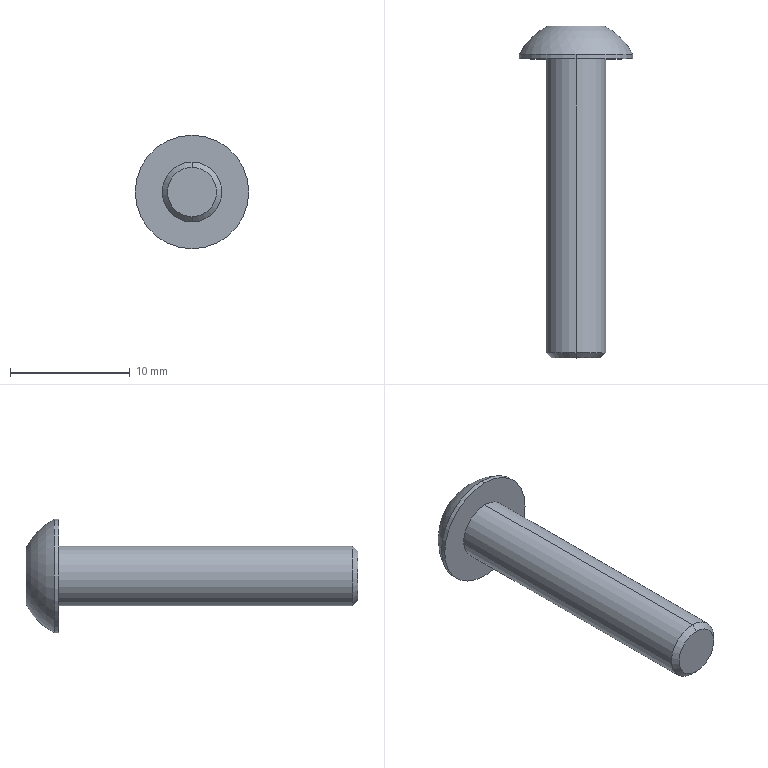Part | SolidWorks | features BaseBody 1 | 1 solid | 17 faces | box 9.5 x 27.75 x 9.5 mm | volume 615.577 mm3 | plane 10 | cylinder 4 | cone 2 | sphere 1 | commonest cylinder face diameters 5 x2 9.5 x2
STEP:
#1=CARTESIAN_POINT('',(0.,-25.,-2.055));
#2=VERTEX_POINT('',#1);
#3=CARTESIAN_POINT('',(0.,-25.,2.055));
#4=VERTEX_POINT('',#3);
#5=CARTESIAN_POINT('',(0.,-25.,0.));
#6=DIRECTION('',(0.,-1.,0.));
#7=DIRECTION('',(0.,0.,-1.));
#8=AXIS2_PLACEMENT_3D('',#5,#6,#7);
#9=CIRCLE('',#8,2.055);
#10=EDGE_CURVE('',#2,#4,#9,.T.);
#11=ORIENTED_EDGE('',*,*,#10,.F.);
#12=CARTESIAN_POINT('',(0.,-24.555,-2.5));
#13=VERTEX_POINT('',#12);
#14=CARTESIAN_POINT('',(0.,-25.,-2.055));
#15=DIRECTION('',(0.,0.7071,-0.7071));
#16=VECTOR('',#15,1000.);
#17=LINE('',#14,#16);
#18=EDGE_CURVE('',#2,#13,#17,.T.);
#19=ORIENTED_EDGE('',*,*,#18,.T.);
#20=CARTESIAN_POINT('',(0.,-24.555,2.5));
#21=VERTEX_POINT('',#20);
#22=CARTESIAN_POINT('',(0.,-24.555,0.));
#23=DIRECTION('',(0.,1.,0.));
#24=DIRECTION('',(0.,0.,-1.));
#25=AXIS2_PLACEMENT_3D('',#22,#23,#24);
#26=CIRCLE('',#25,2.5);
#27=EDGE_CURVE('',#21,#13,#26,.T.);
#28=ORIENTED_EDGE('',*,*,#27,.F.);
#29=CARTESIAN_POINT('',(0.,-25.,2.055));
#30=DIRECTION('',(0.,0.7071,0.7071));
#31=VECTOR('',#30,1000.);
#32=LINE('',#29,#31);
#33=EDGE_CURVE('',#4,#21,#32,.T.);
#34=ORIENTED_EDGE('',*,*,#33,.F.);
#35=EDGE_LOOP('',(#11,#19,#28,#34));
#36=FACE_OUTER_BOUND('',#35,.T.);
#37=CARTESIAN_POINT('',(0.,-25.,0.));
#38=DIRECTION('',(0.,1.,0.));
#39=DIRECTION('',(0.,0.,1.));
#40=AXIS2_PLACEMENT_3D('',#37,#38,#39);
#41=CONICAL_SURFACE('',#40,2.055,0.7854);
#42=ADVANCED_FACE('',(#36),#41,.T.);
#43=ORIENTED_EDGE('',*,*,#27,.T.);
#44=CARTESIAN_POINT('',(0.,0.,-2.5));
#45=VERTEX_POINT('',#44);
#46=CARTESIAN_POINT('',(0.,-25.,-2.5));
#47=DIRECTION('',(0.,1.,0.));
#48=VECTOR('',#47,1000.);
#49=LINE('',#46,#48);
#50=EDGE_CURVE('',#13,#45,#49,.T.);
#51=ORIENTED_EDGE('',*,*,#50,.T.);
#52=CARTESIAN_POINT('',(0.,0.,2.5));
#53=VERTEX_POINT('',#52);
#54=CARTESIAN_POINT('',(0.,0.,0.));
#55=DIRECTION('',(0.,-1.,0.));
#56=DIRECTION('',(0.,0.,1.));
#57=AXIS2_PLACEMENT_3D('',#54,#55,#56);
#58=CIRCLE('',#57,2.5);
#59=EDGE_CURVE('',#45,#53,#58,.T.);
#60=ORIENTED_EDGE('',*,*,#59,.T.);
#61=CARTESIAN_POINT('',(0.,-25.,2.5));
#62=DIRECTION('',(0.,1.,0.));
#63=VECTOR('',#62,1000.);
#64=LINE('',#61,#63);
#65=EDGE_CURVE('',#21,#53,#64,.T.);
#66=ORIENTED_EDGE('',*,*,#65,.F.);
#67=EDGE_LOOP('',(#43,#51,#60,#66));
#68=FACE_OUTER_BOUND('',#67,.T.);
#69=CARTESIAN_POINT('',(0.,-25.,0.));
#70=DIRECTION('',(0.,1.,0.));
#71=DIRECTION('',(0.,0.,1.));
#72=AXIS2_PLACEMENT_3D('',#69,#70,#71);
#73=CYLINDRICAL_SURFACE('',#72,2.5);
#74=ADVANCED_FACE('',(#68),#73,.T.);
#75=CARTESIAN_POINT('',(0.,0.38,-4.75));
#76=VERTEX_POINT('',#75);
#77=CARTESIAN_POINT('',(0.,0.38,4.75));
#78=VERTEX_POINT('',#77);
#79=CARTESIAN_POINT('',(0.,0.38,0.));
#80=DIRECTION('',(0.,-1.,0.));
#81=DIRECTION('',(0.,0.,-1.));
#82=AXIS2_PLACEMENT_3D('',#79,#80,#81);
#83=CIRCLE('',#82,4.75);
#84=EDGE_CURVE('',#76,#78,#83,.T.);
#85=ORIENTED_EDGE('',*,*,#84,.T.);
#86=CARTESIAN_POINT('',(0.,0.,4.75));
#87=VERTEX_POINT('',#86);
#88=CARTESIAN_POINT('',(0.,2.75,4.75));
#89=DIRECTION('',(0.,-1.,0.));
#90=VECTOR('',#89,1000.);
#91=LINE('',#88,#90);
#92=EDGE_CURVE('',#78,#87,#91,.T.);
#93=ORIENTED_EDGE('',*,*,#92,.T.);
#94=CARTESIAN_POINT('',(0.,0.,-4.75));
#95=VERTEX_POINT('',#94);
#96=CARTESIAN_POINT('',(0.,0.,0.));
#97=DIRECTION('',(0.,1.,0.));
#98=DIRECTION('',(0.,0.,1.));
#99=AXIS2_PLACEMENT_3D('',#96,#97,#98);
#100=CIRCLE('',#99,4.75);
#101=EDGE_CURVE('',#87,#95,#100,.T.);
#102=ORIENTED_EDGE('',*,*,#101,.T.);
#103=CARTESIAN_POINT('',(0.,2.75,-4.75));
#104=DIRECTION('',(0.,-1.,0.));
#105=VECTOR('',#104,1000.);
#106=LINE('',#103,#105);
#107=EDGE_CURVE('',#76,#95,#106,.T.);
#108=ORIENTED_EDGE('',*,*,#107,.F.);
#109=EDGE_LOOP('',(#85,#93,#102,#108));
#110=FACE_OUTER_BOUND('',#109,.T.);
#111=CARTESIAN_POINT('',(0.,2.75,0.));
#112=DIRECTION('',(0.,-1.,0.));
#113=DIRECTION('',(0.,0.,-1.));
#114=AXIS2_PLACEMENT_3D('',#111,#112,#113);
#115=CYLINDRICAL_SURFACE('',#114,4.75);
#116=ADVANCED_FACE('',(#110),#115,.T.);
#117=CARTESIAN_POINT('',(0.8862,2.75,1.535));
#118=VERTEX_POINT('',#117);
#119=CARTESIAN_POINT('',(1.772,2.75,0.));
#120=VERTEX_POINT('',#119);
#121=CARTESIAN_POINT('',(0.8862,2.75,1.535));
#122=DIRECTION('',(0.5,0.,-0.866));
#123=VECTOR('',#122,1000.);
#124=LINE('',#121,#123);
#125=EDGE_CURVE('',#118,#120,#124,.T.);
#126=ORIENTED_EDGE('',*,*,#125,.F.);
#127=CARTESIAN_POINT('',(-0.8862,2.75,1.535));
#128=VERTEX_POINT('',#127);
#129=CARTESIAN_POINT('',(-0.8862,2.75,1.535));
#130=DIRECTION('',(1.,0.,0.));
#131=VECTOR('',#130,1000.);
#132=LINE('',#129,#131);
#133=EDGE_CURVE('',#128,#118,#132,.T.);
#134=ORIENTED_EDGE('',*,*,#133,.F.);
#135=CARTESIAN_POINT('',(-1.772,2.75,0.));
#136=VERTEX_POINT('',#135);
#137=CARTESIAN_POINT('',(-1.772,2.75,0.));
#138=DIRECTION('',(0.5,0.,0.866));
#139=VECTOR('',#138,1000.);
#140=LINE('',#137,#139);
#141=EDGE_CURVE('',#136,#128,#140,.T.);
#142=ORIENTED_EDGE('',*,*,#141,.F.);
#143=CARTESIAN_POINT('',(-0.8862,2.75,-1.535));
#144=VERTEX_POINT('',#143);
#145=CARTESIAN_POINT('',(-0.8862,2.75,-1.535));
#146=DIRECTION('',(-0.5,0.,0.866));
#147=VECTOR('',#146,1000.);
#148=LINE('',#145,#147);
#149=EDGE_CURVE('',#144,#136,#148,.T.);
#150=ORIENTED_EDGE('',*,*,#149,.F.);
#151=CARTESIAN_POINT('',(0.8862,2.75,-1.535));
#152=VERTEX_POINT('',#151);
#153=CARTESIAN_POINT('',(0.8862,2.75,-1.535));
#154=DIRECTION('',(-1.,0.,0.));
#155=VECTOR('',#154,1000.);
#156=LINE('',#153,#155);
#157=EDGE_CURVE('',#152,#144,#156,.T.);
#158=ORIENTED_EDGE('',*,*,#157,.F.);
#159=CARTESIAN_POINT('',(1.772,2.75,0.));
#160=DIRECTION('',(-0.5,0.,-0.866));
#161=VECTOR('',#160,1000.);
#162=LINE('',#159,#161);
#163=EDGE_CURVE('',#120,#152,#162,.T.);
#164=ORIENTED_EDGE('',*,*,#163,.F.);
#165=EDGE_LOOP('',(#126,#134,#142,#150,#158,#164));
#166=FACE_BOUND('',#165,.T.);
#167=CARTESIAN_POINT('',(0.,2.75,-2.375));
#168=VERTEX_POINT('',#167);
#169=CARTESIAN_POINT('',(0.,2.75,2.375));
#170=VERTEX_POINT('',#169);
#171=CARTESIAN_POINT('',(0.,2.75,0.));
#172=DIRECTION('',(0.,-1.,0.));
#173=DIRECTION('',(0.,0.,-1.));
#174=AXIS2_PLACEMENT_3D('',#171,#172,#173);
#175=CIRCLE('',#174,2.375);
#176=EDGE_CURVE('',#168,#170,#175,.T.);
#177=ORIENTED_EDGE('',*,*,#176,.F.);
#178=CARTESIAN_POINT('',(0.,2.75,0.));
#179=DIRECTION('',(0.,-1.,0.));
#180=DIRECTION('',(0.,0.,-1.));
#181=AXIS2_PLACEMENT_3D('',#178,#179,#180);
#182=CIRCLE('',#181,2.375);
#183=EDGE_CURVE('',#170,#168,#182,.T.);
#184=ORIENTED_EDGE('',*,*,#183,.F.);
#185=EDGE_LOOP('',(#177,#184));
#186=FACE_OUTER_BOUND('',#185,.T.);
#187=CARTESIAN_POINT('',(0.,2.75,0.));
#188=DIRECTION('',(0.,1.,0.));
#189=DIRECTION('',(1.,0.,0.));
#190=AXIS2_PLACEMENT_3D('',#187,#188,#189);
#191=PLANE('',#190);
#192=ADVANCED_FACE('',(#166,#186),#191,.T.);
#193=ORIENTED_EDGE('',*,*,#125,.T.);
#194=CARTESIAN_POINT('',(1.772,1.19,0.));
#195=VERTEX_POINT('',#194);
#196=CARTESIAN_POINT('',(1.772,1.19,0.));
#197=DIRECTION('',(0.,1.,0.));
#198=VECTOR('',#197,1000.);
#199=LINE('',#196,#198);
#200=EDGE_CURVE('',#195,#120,#199,.T.);
#201=ORIENTED_EDGE('',*,*,#200,.F.);
#202=CARTESIAN_POINT('',(0.8862,1.19,1.535));
#203=VERTEX_POINT('',#202);
#204=CARTESIAN_POINT('',(0.8862,1.19,1.535));
#205=DIRECTION('',(0.5,0.,-0.866));
#206=VECTOR('',#205,1000.);
#207=LINE('',#204,#206);
#208=EDGE_CURVE('',#203,#195,#207,.T.);
#209=ORIENTED_EDGE('',*,*,#208,.F.);
#210=CARTESIAN_POINT('',(0.8862,1.19,1.535));
#211=DIRECTION('',(0.,1.,0.));
#212=VECTOR('',#211,1000.);
#213=LINE('',#210,#212);
#214=EDGE_CURVE('',#203,#118,#213,.T.);
#215=ORIENTED_EDGE('',*,*,#214,.T.);
#216=EDGE_LOOP('',(#193,#201,#209,#215));
#217=FACE_OUTER_BOUND('',#216,.T.);
#218=CARTESIAN_POINT('',(0.8862,1.19,1.535));
#219=DIRECTION('',(0.866,0.,0.5));
#220=DIRECTION('',(0.,-1.,0.));
#221=AXIS2_PLACEMENT_3D('',#218,#219,#220);
#222=PLANE('',#221);
#223=ADVANCED_FACE('',(#217),#222,.F.);
#224=ORIENTED_EDGE('',*,*,#133,.T.);
#225=ORIENTED_EDGE('',*,*,#214,.F.);
#226=CARTESIAN_POINT('',(-0.8862,1.19,1.535));
#227=VERTEX_POINT('',#226);
#228=CARTESIAN_POINT('',(-0.8862,1.19,1.535));
#229=DIRECTION('',(1.,0.,0.));
#230=VECTOR('',#229,1000.);
#231=LINE('',#228,#230);
#232=EDGE_CURVE('',#227,#203,#231,.T.);
#233=ORIENTED_EDGE('',*,*,#232,.F.);
#234=CARTESIAN_POINT('',(-0.8862,1.19,1.535));
#235=DIRECTION('',(0.,1.,0.));
#236=VECTOR('',#235,1000.);
#237=LINE('',#234,#236);
#238=EDGE_CURVE('',#227,#128,#237,.T.);
#239=ORIENTED_EDGE('',*,*,#238,.T.);
#240=EDGE_LOOP('',(#224,#225,#233,#239));
#241=FACE_OUTER_BOUND('',#240,.T.);
#242=CARTESIAN_POINT('',(-0.8862,1.19,1.535));
#243=DIRECTION('',(0.,0.,1.));
#244=DIRECTION('',(1.,0.,0.));
#245=AXIS2_PLACEMENT_3D('',#242,#243,#244);
#246=PLANE('',#245);
#247=ADVANCED_FACE('',(#241),#246,.F.);
#248=ORIENTED_EDGE('',*,*,#141,.T.);
#249=ORIENTED_EDGE('',*,*,#238,.F.);
#250=CARTESIAN_POINT('',(-1.772,1.19,0.));
#251=VERTEX_POINT('',#250);
#252=CARTESIAN_POINT('',(-1.772,1.19,0.));
#253=DIRECTION('',(0.5,0.,0.866));
#254=VECTOR('',#253,1000.);
#255=LINE('',#252,#254);
#256=EDGE_CURVE('',#251,#227,#255,.T.);
#257=ORIENTED_EDGE('',*,*,#256,.F.);
#258=CARTESIAN_POINT('',(-1.772,1.19,0.));
#259=DIRECTION('',(0.,1.,0.));
#260=VECTOR('',#259,1000.);
#261=LINE('',#258,#260);
#262=EDGE_CURVE('',#251,#136,#261,.T.);
#263=ORIENTED_EDGE('',*,*,#262,.T.);
#264=EDGE_LOOP('',(#248,#249,#257,#263));
#265=FACE_OUTER_BOUND('',#264,.T.);
#266=CARTESIAN_POINT('',(-1.772,1.19,0.));
#267=DIRECTION('',(-0.866,0.,0.5));
#268=DIRECTION('',(0.,1.,0.));
#269=AXIS2_PLACEMENT_3D('',#266,#267,#268);
#270=PLANE('',#269);
#271=ADVANCED_FACE('',(#265),#270,.F.);
#272=ORIENTED_EDGE('',*,*,#149,.T.);
#273=ORIENTED_EDGE('',*,*,#262,.F.);
#274=CARTESIAN_POINT('',(-0.8862,1.19,-1.535));
#275=VERTEX_POINT('',#274);
#276=CARTESIAN_POINT('',(-0.8862,1.19,-1.535));
#277=DIRECTION('',(-0.5,0.,0.866));
#278=VECTOR('',#277,1000.);
#279=LINE('',#276,#278);
#280=EDGE_CURVE('',#275,#251,#279,.T.);
#281=ORIENTED_EDGE('',*,*,#280,.F.);
#282=CARTESIAN_POINT('',(-0.8862,1.19,-1.535));
#283=DIRECTION('',(0.,1.,0.));
#284=VECTOR('',#283,1000.);
#285=LINE('',#282,#284);
#286=EDGE_CURVE('',#275,#144,#285,.T.);
#287=ORIENTED_EDGE('',*,*,#286,.T.);
#288=EDGE_LOOP('',(#272,#273,#281,#287));
#289=FACE_OUTER_BOUND('',#288,.T.);
#290=CARTESIAN_POINT('',(-0.8862,1.19,-1.535));
#291=DIRECTION('',(-0.866,0.,-0.5));
#292=DIRECTION('',(-0.5,0.,0.866));
#293=AXIS2_PLACEMENT_3D('',#290,#291,#292);
#294=PLANE('',#293);
#295=ADVANCED_FACE('',(#289),#294,.F.);
#296=ORIENTED_EDGE('',*,*,#157,.T.);
#297=ORIENTED_EDGE('',*,*,#286,.F.);
#298=CARTESIAN_POINT('',(0.8862,1.19,-1.535));
#299=VERTEX_POINT('',#298);
#300=CARTESIAN_POINT('',(0.8862,1.19,-1.535));
#301=DIRECTION('',(-1.,0.,0.));
#302=VECTOR('',#301,1000.);
#303=LINE('',#300,#302);
#304=EDGE_CURVE('',#299,#275,#303,.T.);
#305=ORIENTED_EDGE('',*,*,#304,.F.);
#306=CARTESIAN_POINT('',(0.8862,1.19,-1.535));
#307=DIRECTION('',(0.,1.,0.));
#308=VECTOR('',#307,1000.);
#309=LINE('',#306,#308);
#310=EDGE_CURVE('',#299,#152,#309,.T.);
#311=ORIENTED_EDGE('',*,*,#310,.T.);
#312=EDGE_LOOP('',(#296,#297,#305,#311));
#313=FACE_OUTER_BOUND('',#312,.T.);
#314=CARTESIAN_POINT('',(0.8862,1.19,-1.535));
#315=DIRECTION('',(0.,0.,-1.));
#316=DIRECTION('',(-1.,0.,0.));
#317=AXIS2_PLACEMENT_3D('',#314,#315,#316);
#318=PLANE('',#317);
#319=ADVANCED_FACE('',(#313),#318,.F.);
#320=ORIENTED_EDGE('',*,*,#163,.T.);
#321=ORIENTED_EDGE('',*,*,#310,.F.);
#322=CARTESIAN_POINT('',(1.772,1.19,0.));
#323=DIRECTION('',(-0.5,0.,-0.866));
#324=VECTOR('',#323,1000.);
#325=LINE('',#322,#324);
#326=EDGE_CURVE('',#195,#299,#325,.T.);
#327=ORIENTED_EDGE('',*,*,#326,.F.);
#328=ORIENTED_EDGE('',*,*,#200,.T.);
#329=EDGE_LOOP('',(#320,#321,#327,#328));
#330=FACE_OUTER_BOUND('',#329,.T.);
#331=CARTESIAN_POINT('',(1.772,1.19,0.));
#332=DIRECTION('',(0.866,0.,-0.5));
#333=DIRECTION('',(0.,-1.,0.));
#334=AXIS2_PLACEMENT_3D('',#331,#332,#333);
#335=PLANE('',#334);
#336=ADVANCED_FACE('',(#330),#335,.F.);
#337=ORIENTED_EDGE('',*,*,#208,.T.);
#338=ORIENTED_EDGE('',*,*,#326,.T.);
#339=ORIENTED_EDGE('',*,*,#304,.T.);
#340=ORIENTED_EDGE('',*,*,#280,.T.);
#341=ORIENTED_EDGE('',*,*,#256,.T.);
#342=ORIENTED_EDGE('',*,*,#232,.T.);
#343=EDGE_LOOP('',(#337,#338,#339,#340,#341,#342));
#344=FACE_OUTER_BOUND('',#343,.T.);
#345=CARTESIAN_POINT('',(0.,1.19,0.));
#346=DIRECTION('',(0.,1.,0.));
#347=DIRECTION('',(1.,0.,0.));
#348=AXIS2_PLACEMENT_3D('',#345,#346,#347);
#349=PLANE('',#348);
#350=ADVANCED_FACE('',(#344),#349,.T.);
#351=CARTESIAN_POINT('',(0.,-25.,0.));
#352=DIRECTION('',(0.,-1.,0.));
#353=DIRECTION('',(0.,0.,-1.));
#354=AXIS2_PLACEMENT_3D('',#351,#352,#353);
#355=CIRCLE('',#354,2.055);
#356=EDGE_CURVE('',#4,#2,#355,.T.);
#357=ORIENTED_EDGE('',*,*,#356,.T.);
#358=ORIENTED_EDGE('',*,*,#10,.T.);
#359=EDGE_LOOP('',(#357,#358));
#360=FACE_OUTER_BOUND('',#359,.T.);
#361=CARTESIAN_POINT('',(0.,-25.,0.));
#362=DIRECTION('',(0.,-1.,0.));
#363=DIRECTION('',(0.,0.,-1.));
#364=AXIS2_PLACEMENT_3D('',#361,#362,#363);
#365=PLANE('',#364);
#366=ADVANCED_FACE('',(#360),#365,.T.);
#367=CARTESIAN_POINT('',(0.,0.,0.));
#368=DIRECTION('',(0.,-1.,0.));
#369=DIRECTION('',(0.,0.,1.));
#370=AXIS2_PLACEMENT_3D('',#367,#368,#369);
#371=CIRCLE('',#370,2.5);
#372=EDGE_CURVE('',#53,#45,#371,.T.);
#373=ORIENTED_EDGE('',*,*,#372,.F.);
#374=ORIENTED_EDGE('',*,*,#59,.F.);
#375=EDGE_LOOP('',(#373,#374));
#376=FACE_BOUND('',#375,.T.);
#377=CARTESIAN_POINT('',(0.,0.,0.));
#378=DIRECTION('',(0.,1.,0.));
#379=DIRECTION('',(0.,0.,1.));
#380=AXIS2_PLACEMENT_3D('',#377,#378,#379);
#381=CIRCLE('',#380,4.75);
#382=EDGE_CURVE('',#95,#87,#381,.T.);
#383=ORIENTED_EDGE('',*,*,#382,.F.);
#384=ORIENTED_EDGE('',*,*,#101,.F.);
#385=EDGE_LOOP('',(#383,#384));
#386=FACE_OUTER_BOUND('',#385,.T.);
#387=CARTESIAN_POINT('',(0.,0.,0.));
#388=DIRECTION('',(0.,1.,0.));
#389=DIRECTION('',(1.,0.,0.));
#390=AXIS2_PLACEMENT_3D('',#387,#388,#389);
#391=PLANE('',#390);
#392=ADVANCED_FACE('',(#376,#386),#391,.F.);
#393=ORIENTED_EDGE('',*,*,#92,.F.);
#394=CARTESIAN_POINT('',(0.,0.38,0.));
#395=DIRECTION('',(0.,-1.,0.));
#396=DIRECTION('',(0.,0.,-1.));
#397=AXIS2_PLACEMENT_3D('',#394,#395,#396);
#398=CIRCLE('',#397,4.75);
#399=EDGE_CURVE('',#78,#76,#398,.T.);
#400=ORIENTED_EDGE('',*,*,#399,.T.);
#401=ORIENTED_EDGE('',*,*,#107,.T.);
#402=ORIENTED_EDGE('',*,*,#382,.T.);
#403=EDGE_LOOP('',(#393,#400,#401,#402));
#404=FACE_OUTER_BOUND('',#403,.T.);
#405=CARTESIAN_POINT('',(0.,2.75,0.));
#406=DIRECTION('',(0.,-1.,0.));
#407=DIRECTION('',(0.,0.,-1.));
#408=AXIS2_PLACEMENT_3D('',#405,#406,#407);
#409=CYLINDRICAL_SURFACE('',#408,4.75);
#410=ADVANCED_FACE('',(#404),#409,.T.);
#411=ORIENTED_EDGE('',*,*,#50,.F.);
#412=CARTESIAN_POINT('',(0.,-24.555,0.));
#413=DIRECTION('',(0.,1.,0.));
#414=DIRECTION('',(0.,0.,-1.));
#415=AXIS2_PLACEMENT_3D('',#412,#413,#414);
#416=CIRCLE('',#415,2.5);
#417=EDGE_CURVE('',#13,#21,#416,.T.);
#418=ORIENTED_EDGE('',*,*,#417,.T.);
#419=ORIENTED_EDGE('',*,*,#65,.T.);
#420=ORIENTED_EDGE('',*,*,#372,.T.);
#421=EDGE_LOOP('',(#411,#418,#419,#420));
#422=FACE_OUTER_BOUND('',#421,.T.);
#423=CARTESIAN_POINT('',(0.,-25.,0.));
#424=DIRECTION('',(0.,1.,0.));
#425=DIRECTION('',(0.,0.,1.));
#426=AXIS2_PLACEMENT_3D('',#423,#424,#425);
#427=CYLINDRICAL_SURFACE('',#426,2.5);
#428=ADVANCED_FACE('',(#422),#427,.T.);
#429=ORIENTED_EDGE('',*,*,#84,.F.);
#430=ORIENTED_EDGE('',*,*,#399,.F.);
#431=EDGE_LOOP('',(#429,#430));
#432=FACE_OUTER_BOUND('',#431,.T.);
#433=ORIENTED_EDGE('',*,*,#176,.T.);
#434=ORIENTED_EDGE('',*,*,#183,.T.);
#435=EDGE_LOOP('',(#433,#434));
#436=FACE_BOUND('',#435,.T.);
#437=CARTESIAN_POINT('',(0.,-2.005,0.));
#438=DIRECTION('',(0.,1.,0.));
#439=DIRECTION('',(1.,0.,0.));
#440=AXIS2_PLACEMENT_3D('',#437,#438,#439);
#441=SPHERICAL_SURFACE('',#440,5.315);
#442=ADVANCED_FACE('',(#432,#436),#441,.T.);
#443=ORIENTED_EDGE('',*,*,#18,.F.);
#444=ORIENTED_EDGE('',*,*,#356,.F.);
#445=ORIENTED_EDGE('',*,*,#33,.T.);
#446=ORIENTED_EDGE('',*,*,#417,.F.);
#447=EDGE_LOOP('',(#443,#444,#445,#446));
#448=FACE_OUTER_BOUND('',#447,.T.);
#449=CARTESIAN_POINT('',(0.,-25.,0.));
#450=DIRECTION('',(0.,1.,0.));
#451=DIRECTION('',(0.,0.,1.));
#452=AXIS2_PLACEMENT_3D('',#449,#450,#451);
#453=CONICAL_SURFACE('',#452,2.055,0.7854);
#454=ADVANCED_FACE('',(#448),#453,.T.);
#455=CLOSED_SHELL('',(#42,#74,#116,#192,#223,#247,#271,#295,#319,#336,#350,#366,#392,#410,#428,#442,#454));
#456=MANIFOLD_SOLID_BREP('',#455);
#457=CARTESIAN_POINT('',(0.,0.,0.));
#458=DIRECTION('',(0.,0.,1.));
#459=DIRECTION('',(1.,0.,0.));
#460=AXIS2_PLACEMENT_3D('',#457,#458,#459);
#461=(LENGTH_UNIT()NAMED_UNIT(*)SI_UNIT(.MILLI.,.METRE.));
#462=UNCERTAINTY_MEASURE_WITH_UNIT(LENGTH_MEASURE(0.00001),#461,'','');
#463=(NAMED_UNIT(*)PLANE_ANGLE_UNIT()SI_UNIT($,.RADIAN.));
#464=(NAMED_UNIT(*)SI_UNIT($,.STERADIAN.)SOLID_ANGLE_UNIT());
#465=(GEOMETRIC_REPRESENTATION_CONTEXT(3)GLOBAL_UNCERTAINTY_ASSIGNED_CONTEXT((#462))GLOBAL_UNIT_ASSIGNED_CONTEXT((#461,#463,#464))REPRESENTATION_CONTEXT('',''));
#466=ADVANCED_BREP_SHAPE_REPRESENTATION('',(#456,#460),#465);